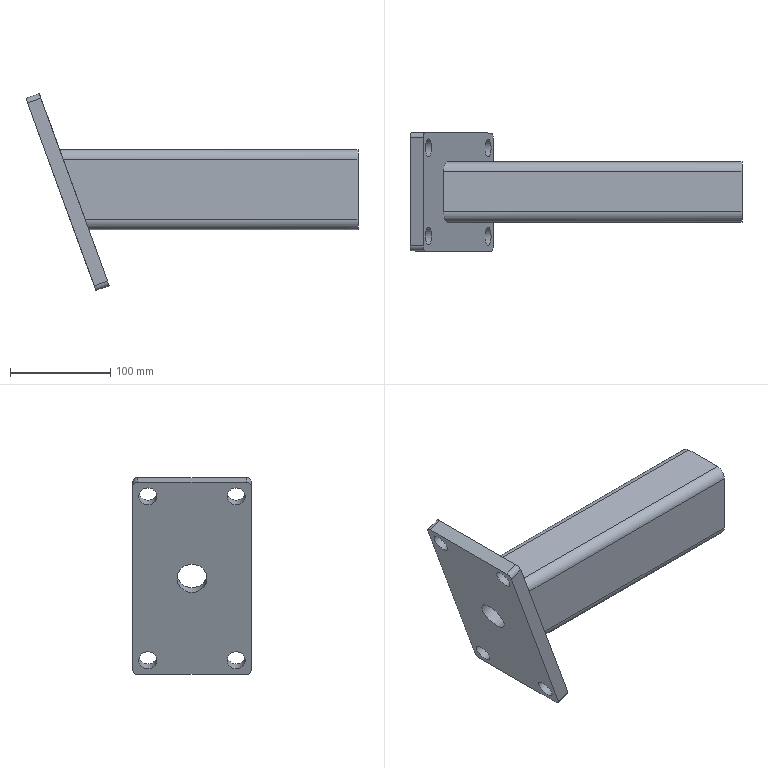Part | STEP file | COMPOUND | 2 solids | 33 faces | box 331.222 x 118 x 196.486 mm | volume 662464 mm3 | cylinder 17 | plane 16 | commonest cylinder face diameters 10 x8 18 x4 20 x4 30 x1